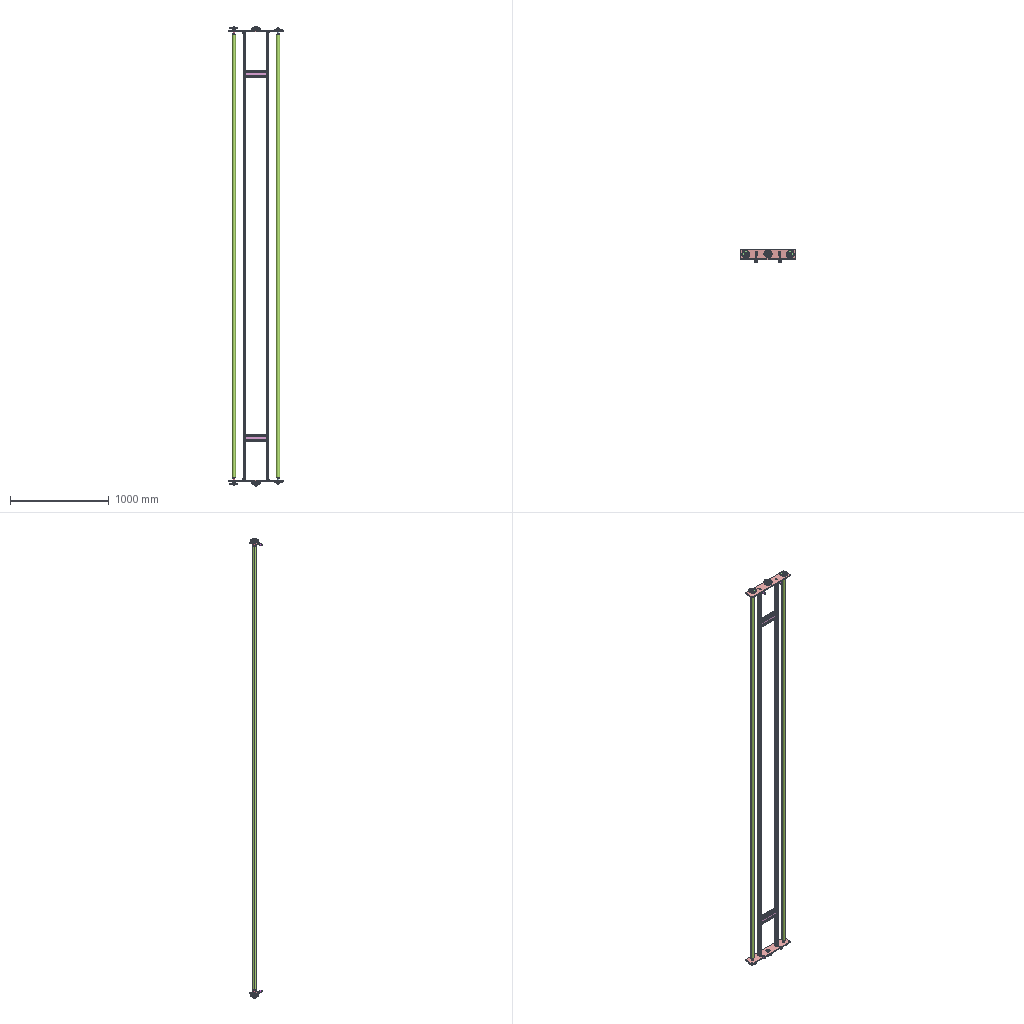Assembly | SolidWorks | 16 different items | 37 placed | box 550 x 134 x 4667 mm
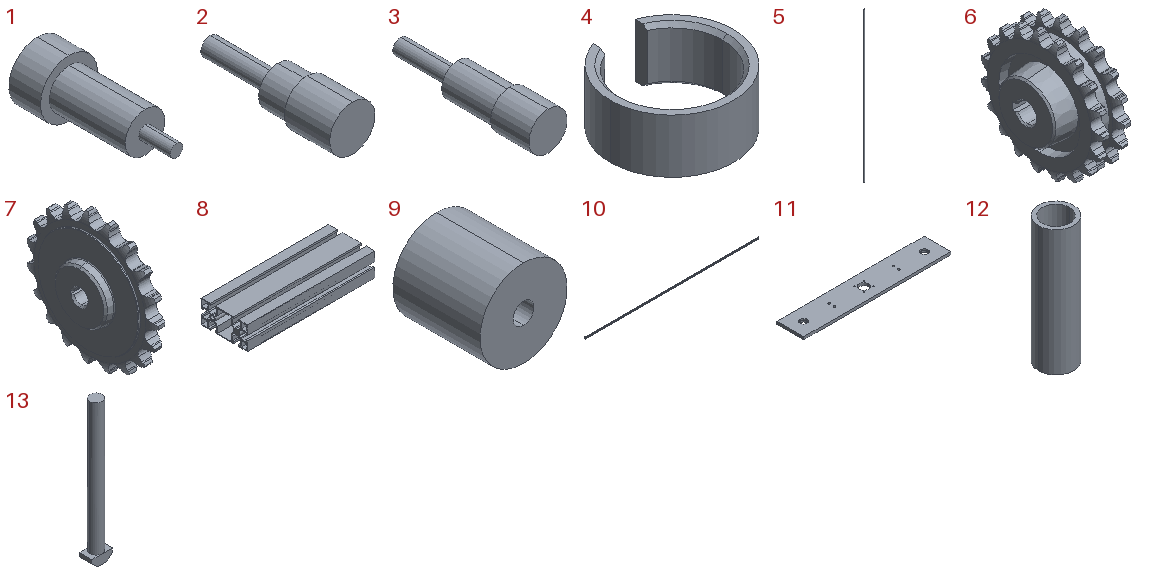Parts list (item | name | quantity | size | volume | features):
1 | - | x2 | 18 x 44 x 18 mm | 5338 mm3 | features ICE 3, Extrusion 1
2 | - | x2 | 20 x 62.8 x 20 mm | 10660 mm3 | features ICE 3, Extrusion 1
3 | - | x2 | 20 x 77.2 x 20 mm | 13929 mm3 | features ICE 3, Extrusion 1
4 | - | x2 | 16 x 15.512 x 7 mm | 385.007 mm3 | features Chamfer 1, Extrusion 1, ICE 1
5 | - | x2 | 35 x 35 x 4500 mm | 1357168 mm3 | features Extrusion 1
6 | - | x2 | 40 x 81.595 x 81.862 mm | 92773 mm3 | features Cut 2, Revolution 2, Chamfer 1, CirPattern 1, LPattern 1
7 | - | x4 | 20 x 81.595 x 81.862 mm | 45176 mm3 | features Cut 2, Revolution 2, Chamfer 1, CirPattern 1, Fillet 1, MirrorPattern 1
8 | - | x2 | 220 x 80 x 40 mm | 163035 mm3 | features WeldMemberFeat 1, WeldmentFeature 1
9 | - | x4 | 25 x 25 x 25 mm | 11565 mm3 | features Extrusion 1
10 | - | x2 | 4546 x 20 x 40 mm | 1364953 mm3 | features HoleWzd 1, WeldMemberFeat 1, WeldmentFeature 1
11 | - | x2 | 550 x 100 x 10 mm | 528570 mm3 | features ICE 5, Extrusion 1, Fillet 1, HoleWzd 1, MirrorPattern 1
12 | - | x4 | 9 x 9 x 32 mm | 804.248 mm3 | features Extrusion 1
13 | - | x4 | 10 x 6 x 69.5 mm | 2064 mm3 | features Extrusion 1, ICE 1
14 | deep groove ball bearings gb | x1 | - | - | -
15 | hex nuts 1-fine pitch-grades ab gb | x1 | - | - | -
16 | Brush Outer Diameter | x1 | - | - | -
Mates (type | each side: item.copy, entity, surface, feature):
Coincident | 11.1 face plane Boss-Extrude1 | 10.1 face plane Aluminum profile 20 X 40 X R1.5(1)
Symmetric | 11.1 face plane Boss-Extrude1 | 11.1 face plane Boss-Extrude1 | 5.1 plane
Coincident | 10.2 face plane Aluminum profile 20 X 40 X R1.5(1) | 8.1 face plane Aluminum profile 40 X 80L X R0.3(1) | 2 times
Concentric | assembly face | 11.2 face cylinder Cut-Extrude2
Symmetric | 11.1 plane | 10.1 face plane Aluminum profile 20 X 40 X R1.5(1) | 10.1 face plane Aluminum profile 20 X 40 X R1.5(1)
DistanceDim | 10.1 face plane Aluminum profile 20 X 40 X R1.5(1) | 11.1 plane
Concentric | assembly face | 7.1 face cylinder Revolve1
Coincident | 6.1 plane | 7.2 plane
Coincident | 6.1 plane | 7.1 plane
Coincident | 11.1 face plane Boss-Extrude1 | 11.2 face plane Boss-Extrude1 | 2 times
Concentric | assembly face | 2.1 face cylinder Boss-Extrude1
Parallel | 10.1 face plane Aluminum profile 20 X 40 X R1.5(1) | 13.1 face plane Boss-Extrude1
Coincident | 10.1 face plane Aluminum profile 20 X 40 X R1.5(1) | 13.1 face plane Boss-Extrude1
Symmetric | 10.1 face plane Aluminum profile 20 X 40 X R1.5(1) | 10.1 face plane Aluminum profile 20 X 40 X R1.5(1) | 13.1 plane
DistanceDim | 13.1 face plane Boss-Extrude1 | 10.1 face plane Aluminum profile 20 X 40 X R1.5(1)
Concentric | 13.1 face cylinder Boss-Extrude2 | 9.1 face cylinder Boss-Extrude1
Concentric | 13.1 face cylinder Boss-Extrude2 | 12.1 face cylinder Boss-Extrude1
Coincident | 10.1 face plane Aluminum profile 20 X 40 X R1.5(1) | 12.1 face plane Boss-Extrude1
Coincident | 9.1 face plane Boss-Extrude1 | 12.1 face plane Boss-Extrude1
Concentric | 6.1 face cylinder Revolve2 | 1.1 face cylinder Boss-Extrude2
Coincident | 6.1 face plane Revolve2 | 1.1 face plane Boss-Extrude3
Coincident | 6.2 face plane Revolve2 | 1.2 face plane Boss-Extrude3
Concentric | 6.2 face cylinder Revolve2 | 1.2 face cylinder Boss-Extrude2
Coincident | 6.1 face plane Revolve2 | 4.1 face plane Boss-Extrude1